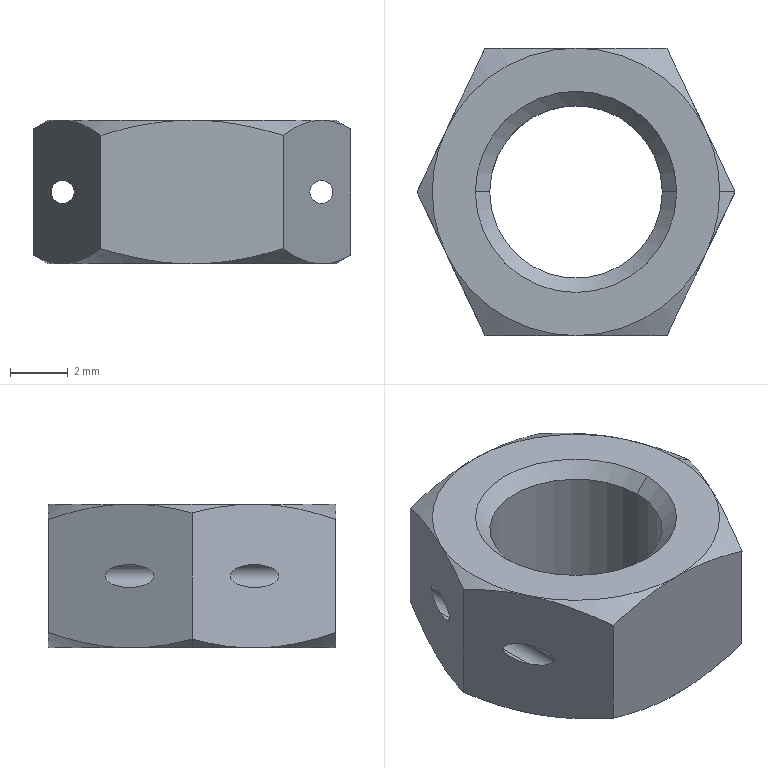Part | SolidWorks | features BaseBody 1 | 1 solid | 30 faces | box 11.062 x 10 x 5 mm | volume 284.112 mm3 | cone 16 | plane 8 | cylinder 6 | commonest cylinder face diameters 0.8 x4 6 x2
STEP:
#1=CARTESIAN_POINT('',(11.537,-31.104,-201.55));
#2=VERTEX_POINT('',#1);
#3=CARTESIAN_POINT('',(11.057,-28.966,-201.55));
#4=VERTEX_POINT('',#3);
#5=CARTESIAN_POINT('',(6.537,-31.104,-201.55));
#6=DIRECTION('',(0.,0.,1.));
#7=DIRECTION('',(-1.,0.,0.));
#8=AXIS2_PLACEMENT_3D('',#5,#6,#7);
#9=CIRCLE('',#8,5.);
#10=EDGE_CURVE('',#2,#4,#9,.T.);
#11=ORIENTED_EDGE('',*,*,#10,.F.);
#12=CARTESIAN_POINT('',(12.068,-31.104,-201.856));
#13=VERTEX_POINT('',#12);
#14=CARTESIAN_POINT('',(11.537,-31.104,-201.55));
#15=DIRECTION('',(0.866,0.,-0.5));
#16=VECTOR('',#15,1000.);
#17=LINE('',#14,#16);
#18=EDGE_CURVE('',#2,#13,#17,.T.);
#19=ORIENTED_EDGE('',*,*,#18,.T.);
#20=CARTESIAN_POINT('',(12.068,-31.104,-201.856));
#21=CARTESIAN_POINT('',(11.736,-30.402,-201.665));
#22=CARTESIAN_POINT('',(11.4,-29.691,-201.55));
#23=CARTESIAN_POINT('',(11.057,-28.966,-201.55));
#24=B_SPLINE_CURVE_WITH_KNOTS('',3,(#20,#21,#22,#23),.UNSPECIFIED.,.F.,.F.,(4,4),(0.,0.002384),.UNSPECIFIED.);
#25=EDGE_CURVE('',#13,#4,#24,.T.);
#26=ORIENTED_EDGE('',*,*,#25,.T.);
#27=EDGE_LOOP('',(#11,#19,#26));
#28=FACE_OUTER_BOUND('',#27,.T.);
#29=CARTESIAN_POINT('',(6.537,-31.104,-201.55));
#30=DIRECTION('',(0.,0.,-1.));
#31=DIRECTION('',(1.,0.,0.));
#32=AXIS2_PLACEMENT_3D('',#29,#30,#31);
#33=CONICAL_SURFACE('',#32,5.,1.047);
#34=ADVANCED_FACE('',(#28),#33,.T.);
#35=CARTESIAN_POINT('',(2.017,-28.966,-206.55));
#36=VERTEX_POINT('',#35);
#37=CARTESIAN_POINT('',(1.537,-31.104,-206.55));
#38=VERTEX_POINT('',#37);
#39=CARTESIAN_POINT('',(6.537,-31.104,-206.55));
#40=DIRECTION('',(0.,0.,1.));
#41=DIRECTION('',(-1.,0.,0.));
#42=AXIS2_PLACEMENT_3D('',#39,#40,#41);
#43=CIRCLE('',#42,5.);
#44=EDGE_CURVE('',#36,#38,#43,.T.);
#45=ORIENTED_EDGE('',*,*,#44,.T.);
#46=CARTESIAN_POINT('',(1.006,-31.104,-206.244));
#47=VERTEX_POINT('',#46);
#48=CARTESIAN_POINT('',(1.537,-31.104,-206.55));
#49=DIRECTION('',(-0.866,0.,0.5));
#50=VECTOR('',#49,1000.);
#51=LINE('',#48,#50);
#52=EDGE_CURVE('',#38,#47,#51,.T.);
#53=ORIENTED_EDGE('',*,*,#52,.T.);
#54=CARTESIAN_POINT('',(1.006,-31.104,-206.244));
#55=CARTESIAN_POINT('',(1.338,-30.402,-206.435));
#56=CARTESIAN_POINT('',(1.674,-29.691,-206.55));
#57=CARTESIAN_POINT('',(2.017,-28.966,-206.55));
#58=B_SPLINE_CURVE_WITH_KNOTS('',3,(#54,#55,#56,#57),.UNSPECIFIED.,.F.,.F.,(4,4),(0.,0.002384),.UNSPECIFIED.);
#59=EDGE_CURVE('',#47,#36,#58,.T.);
#60=ORIENTED_EDGE('',*,*,#59,.T.);
#61=EDGE_LOOP('',(#45,#53,#60));
#62=FACE_OUTER_BOUND('',#61,.T.);
#63=CARTESIAN_POINT('',(6.537,-31.104,-206.55));
#64=DIRECTION('',(0.,0.,1.));
#65=DIRECTION('',(-1.,0.,0.));
#66=AXIS2_PLACEMENT_3D('',#63,#64,#65);
#67=CONICAL_SURFACE('',#66,5.,1.047);
#68=ADVANCED_FACE('',(#62),#67,.T.);
#69=CARTESIAN_POINT('',(9.537,-31.104,-206.55));
#70=VERTEX_POINT('',#69);
#71=CARTESIAN_POINT('',(3.537,-31.104,-206.55));
#72=VERTEX_POINT('',#71);
#73=CARTESIAN_POINT('',(6.537,-31.104,-206.55));
#74=DIRECTION('',(0.,0.,-1.));
#75=DIRECTION('',(-1.,0.,0.));
#76=AXIS2_PLACEMENT_3D('',#73,#74,#75);
#77=CIRCLE('',#76,3.);
#78=EDGE_CURVE('',#70,#72,#77,.T.);
#79=ORIENTED_EDGE('',*,*,#78,.T.);
#80=CARTESIAN_POINT('',(3.537,-31.104,-202.05));
#81=VERTEX_POINT('',#80);
#82=CARTESIAN_POINT('',(3.537,-31.104,-211.55));
#83=DIRECTION('',(0.,0.,1.));
#84=VECTOR('',#83,1000.);
#85=LINE('',#82,#84);
#86=EDGE_CURVE('',#72,#81,#85,.T.);
#87=ORIENTED_EDGE('',*,*,#86,.T.);
#88=CARTESIAN_POINT('',(9.537,-31.104,-202.05));
#89=VERTEX_POINT('',#88);
#90=CARTESIAN_POINT('',(6.537,-31.104,-202.05));
#91=DIRECTION('',(0.,0.,1.));
#92=DIRECTION('',(-1.,0.,0.));
#93=AXIS2_PLACEMENT_3D('',#90,#91,#92);
#94=CIRCLE('',#93,3.);
#95=EDGE_CURVE('',#81,#89,#94,.T.);
#96=ORIENTED_EDGE('',*,*,#95,.T.);
#97=CARTESIAN_POINT('',(9.537,-31.104,-211.55));
#98=DIRECTION('',(0.,0.,1.));
#99=VECTOR('',#98,1000.);
#100=LINE('',#97,#99);
#101=EDGE_CURVE('',#70,#89,#100,.T.);
#102=ORIENTED_EDGE('',*,*,#101,.F.);
#103=EDGE_LOOP('',(#79,#87,#96,#102));
#104=FACE_OUTER_BOUND('',#103,.T.);
#105=CARTESIAN_POINT('',(6.537,-31.104,-211.55));
#106=DIRECTION('',(0.,0.,1.));
#107=DIRECTION('',(1.,0.,0.));
#108=AXIS2_PLACEMENT_3D('',#105,#106,#107);
#109=CYLINDRICAL_SURFACE('',#108,3.);
#110=ADVANCED_FACE('',(#104),#109,.F.);
#111=ORIENTED_EDGE('',*,*,#95,.F.);
#112=CARTESIAN_POINT('',(3.037,-31.104,-201.55));
#113=VERTEX_POINT('',#112);
#114=CARTESIAN_POINT('',(3.537,-31.104,-202.05));
#115=DIRECTION('',(-0.7071,0.,0.7071));
#116=VECTOR('',#115,1000.);
#117=LINE('',#114,#116);
#118=EDGE_CURVE('',#81,#113,#117,.T.);
#119=ORIENTED_EDGE('',*,*,#118,.T.);
#120=CARTESIAN_POINT('',(10.037,-31.104,-201.55));
#121=VERTEX_POINT('',#120);
#122=CARTESIAN_POINT('',(6.537,-31.104,-201.55));
#123=DIRECTION('',(0.,0.,-1.));
#124=DIRECTION('',(-1.,0.,0.));
#125=AXIS2_PLACEMENT_3D('',#122,#123,#124);
#126=CIRCLE('',#125,3.5);
#127=EDGE_CURVE('',#121,#113,#126,.T.);
#128=ORIENTED_EDGE('',*,*,#127,.F.);
#129=CARTESIAN_POINT('',(9.537,-31.104,-202.05));
#130=DIRECTION('',(0.7071,0.,0.7071));
#131=VECTOR('',#130,1000.);
#132=LINE('',#129,#131);
#133=EDGE_CURVE('',#89,#121,#132,.T.);
#134=ORIENTED_EDGE('',*,*,#133,.F.);
#135=EDGE_LOOP('',(#111,#119,#128,#134));
#136=FACE_OUTER_BOUND('',#135,.T.);
#137=CARTESIAN_POINT('',(6.537,-31.104,-202.05));
#138=DIRECTION('',(0.,0.,1.));
#139=DIRECTION('',(1.,0.,0.));
#140=AXIS2_PLACEMENT_3D('',#137,#138,#139);
#141=CONICAL_SURFACE('',#140,3.,0.7854);
#142=ADVANCED_FACE('',(#136),#141,.F.);
#143=CARTESIAN_POINT('',(11.037,-33.284,-204.45));
#144=VERTEX_POINT('',#143);
#145=CARTESIAN_POINT('',(11.037,-33.284,-203.65));
#146=VERTEX_POINT('',#145);
#147=CARTESIAN_POINT('',(11.037,-33.284,-204.45));
#148=CARTESIAN_POINT('',(10.237,-34.976,-204.45));
#149=CARTESIAN_POINT('',(10.237,-34.976,-203.65));
#150=CARTESIAN_POINT('',(11.037,-33.284,-203.65));
#151=(BOUNDED_CURVE()B_SPLINE_CURVE(3,(#147,#148,#149,#150),.UNSPECIFIED.,.F.,.T.)B_SPLINE_CURVE_WITH_KNOTS((4,4),(1.571,4.712),.UNSPECIFIED.)CURVE()GEOMETRIC_REPRESENTATION_ITEM()RATIONAL_B_SPLINE_CURVE((1.,0.3333,0.3333,1.))REPRESENTATION_ITEM(''));
#152=EDGE_CURVE('',#144,#146,#151,.T.);
#153=ORIENTED_EDGE('',*,*,#152,.F.);
#154=CARTESIAN_POINT('',(11.037,-28.924,-204.45));
#155=VERTEX_POINT('',#154);
#156=CARTESIAN_POINT('',(11.037,-36.104,-204.45));
#157=DIRECTION('',(0.,1.,0.));
#158=VECTOR('',#157,1000.);
#159=LINE('',#156,#158);
#160=EDGE_CURVE('',#144,#155,#159,.T.);
#161=ORIENTED_EDGE('',*,*,#160,.T.);
#162=CARTESIAN_POINT('',(11.037,-28.924,-203.65));
#163=VERTEX_POINT('',#162);
#164=CARTESIAN_POINT('',(11.037,-28.924,-203.65));
#165=CARTESIAN_POINT('',(10.237,-27.232,-203.65));
#166=CARTESIAN_POINT('',(10.237,-27.232,-204.45));
#167=CARTESIAN_POINT('',(11.037,-28.924,-204.45));
#168=(BOUNDED_CURVE()B_SPLINE_CURVE(3,(#164,#165,#166,#167),.UNSPECIFIED.,.F.,.T.)B_SPLINE_CURVE_WITH_KNOTS((4,4),(4.712,7.854),.UNSPECIFIED.)CURVE()GEOMETRIC_REPRESENTATION_ITEM()RATIONAL_B_SPLINE_CURVE((1.,0.3333,0.3333,1.))REPRESENTATION_ITEM(''));
#169=EDGE_CURVE('',#163,#155,#168,.T.);
#170=ORIENTED_EDGE('',*,*,#169,.F.);
#171=CARTESIAN_POINT('',(11.037,-36.104,-203.65));
#172=DIRECTION('',(0.,1.,0.));
#173=VECTOR('',#172,1000.);
#174=LINE('',#171,#173);
#175=EDGE_CURVE('',#146,#163,#174,.T.);
#176=ORIENTED_EDGE('',*,*,#175,.F.);
#177=EDGE_LOOP('',(#153,#161,#170,#176));
#178=FACE_OUTER_BOUND('',#177,.T.);
#179=CARTESIAN_POINT('',(11.037,-36.104,-204.05));
#180=DIRECTION('',(0.,1.,0.));
#181=DIRECTION('',(0.,0.,1.));
#182=AXIS2_PLACEMENT_3D('',#179,#180,#181);
#183=CYLINDRICAL_SURFACE('',#182,0.4);
#184=ADVANCED_FACE('',(#178),#183,.F.);
#185=CARTESIAN_POINT('',(2.037,-33.284,-204.45));
#186=VERTEX_POINT('',#185);
#187=CARTESIAN_POINT('',(2.037,-33.284,-203.65));
#188=VERTEX_POINT('',#187);
#189=CARTESIAN_POINT('',(2.037,-33.284,-204.45));
#190=CARTESIAN_POINT('',(1.237,-31.592,-204.45));
#191=CARTESIAN_POINT('',(1.237,-31.592,-203.65));
#192=CARTESIAN_POINT('',(2.037,-33.284,-203.65));
#193=(BOUNDED_CURVE()B_SPLINE_CURVE(3,(#189,#190,#191,#192),.UNSPECIFIED.,.F.,.F.)B_SPLINE_CURVE_WITH_KNOTS((4,4),(4.712,7.854),.UNSPECIFIED.)CURVE()GEOMETRIC_REPRESENTATION_ITEM()RATIONAL_B_SPLINE_CURVE((1.,0.3333,0.3333,1.))REPRESENTATION_ITEM(''));
#194=EDGE_CURVE('',#186,#188,#193,.T.);
#195=ORIENTED_EDGE('',*,*,#194,.F.);
#196=CARTESIAN_POINT('',(2.037,-28.924,-204.45));
#197=VERTEX_POINT('',#196);
#198=CARTESIAN_POINT('',(2.037,-36.104,-204.45));
#199=DIRECTION('',(0.,1.,0.));
#200=VECTOR('',#199,1000.);
#201=LINE('',#198,#200);
#202=EDGE_CURVE('',#186,#197,#201,.T.);
#203=ORIENTED_EDGE('',*,*,#202,.T.);
#204=CARTESIAN_POINT('',(2.037,-28.924,-203.65));
#205=VERTEX_POINT('',#204);
#206=CARTESIAN_POINT('',(2.037,-28.924,-203.65));
#207=CARTESIAN_POINT('',(1.237,-30.616,-203.65));
#208=CARTESIAN_POINT('',(1.237,-30.616,-204.45));
#209=CARTESIAN_POINT('',(2.037,-28.924,-204.45));
#210=(BOUNDED_CURVE()B_SPLINE_CURVE(3,(#206,#207,#208,#209),.UNSPECIFIED.,.F.,.F.)B_SPLINE_CURVE_WITH_KNOTS((4,4),(1.571,4.712),.UNSPECIFIED.)CURVE()GEOMETRIC_REPRESENTATION_ITEM()RATIONAL_B_SPLINE_CURVE((1.,0.3333,0.3333,1.))REPRESENTATION_ITEM(''));
#211=EDGE_CURVE('',#205,#197,#210,.T.);
#212=ORIENTED_EDGE('',*,*,#211,.F.);
#213=CARTESIAN_POINT('',(2.037,-36.104,-203.65));
#214=DIRECTION('',(0.,1.,0.));
#215=VECTOR('',#214,1000.);
#216=LINE('',#213,#215);
#217=EDGE_CURVE('',#188,#205,#216,.T.);
#218=ORIENTED_EDGE('',*,*,#217,.F.);
#219=EDGE_LOOP('',(#195,#203,#212,#218));
#220=FACE_OUTER_BOUND('',#219,.T.);
#221=CARTESIAN_POINT('',(2.037,-36.104,-204.05));
#222=DIRECTION('',(0.,1.,0.));
#223=DIRECTION('',(0.,0.,1.));
#224=AXIS2_PLACEMENT_3D('',#221,#222,#223);
#225=CYLINDRICAL_SURFACE('',#224,0.4);
#226=ADVANCED_FACE('',(#220),#225,.F.);
#227=ORIENTED_EDGE('',*,*,#202,.F.);
#228=CARTESIAN_POINT('',(2.037,-33.284,-203.65));
#229=CARTESIAN_POINT('',(2.837,-34.976,-203.65));
#230=CARTESIAN_POINT('',(2.837,-34.976,-204.45));
#231=CARTESIAN_POINT('',(2.037,-33.284,-204.45));
#232=(BOUNDED_CURVE()B_SPLINE_CURVE(3,(#228,#229,#230,#231),.UNSPECIFIED.,.F.,.F.)B_SPLINE_CURVE_WITH_KNOTS((4,4),(1.571,4.712),.UNSPECIFIED.)CURVE()GEOMETRIC_REPRESENTATION_ITEM()RATIONAL_B_SPLINE_CURVE((1.,0.3333,0.3333,1.))REPRESENTATION_ITEM(''));
#233=EDGE_CURVE('',#188,#186,#232,.T.);
#234=ORIENTED_EDGE('',*,*,#233,.F.);
#235=ORIENTED_EDGE('',*,*,#217,.T.);
#236=CARTESIAN_POINT('',(2.037,-28.924,-204.45));
#237=CARTESIAN_POINT('',(2.837,-27.232,-204.45));
#238=CARTESIAN_POINT('',(2.837,-27.232,-203.65));
#239=CARTESIAN_POINT('',(2.037,-28.924,-203.65));
#240=(BOUNDED_CURVE()B_SPLINE_CURVE(3,(#236,#237,#238,#239),.UNSPECIFIED.,.F.,.F.)B_SPLINE_CURVE_WITH_KNOTS((4,4),(4.712,7.854),.UNSPECIFIED.)CURVE()GEOMETRIC_REPRESENTATION_ITEM()RATIONAL_B_SPLINE_CURVE((1.,0.3333,0.3333,1.))REPRESENTATION_ITEM(''));
#241=EDGE_CURVE('',#197,#205,#240,.T.);
#242=ORIENTED_EDGE('',*,*,#241,.F.);
#243=EDGE_LOOP('',(#227,#234,#235,#242));
#244=FACE_OUTER_BOUND('',#243,.T.);
#245=CARTESIAN_POINT('',(2.037,-36.104,-204.05));
#246=DIRECTION('',(0.,1.,0.));
#247=DIRECTION('',(0.,0.,1.));
#248=AXIS2_PLACEMENT_3D('',#245,#246,#247);
#249=CYLINDRICAL_SURFACE('',#248,0.4);
#250=ADVANCED_FACE('',(#244),#249,.F.);
#251=ORIENTED_EDGE('',*,*,#160,.F.);
#252=CARTESIAN_POINT('',(11.037,-33.284,-203.65));
#253=CARTESIAN_POINT('',(11.837,-31.592,-203.65));
#254=CARTESIAN_POINT('',(11.837,-31.592,-204.45));
#255=CARTESIAN_POINT('',(11.037,-33.284,-204.45));
#256=(BOUNDED_CURVE()B_SPLINE_CURVE(3,(#252,#253,#254,#255),.UNSPECIFIED.,.F.,.T.)B_SPLINE_CURVE_WITH_KNOTS((4,4),(4.712,7.854),.UNSPECIFIED.)CURVE()GEOMETRIC_REPRESENTATION_ITEM()RATIONAL_B_SPLINE_CURVE((1.,0.3333,0.3333,1.))REPRESENTATION_ITEM(''));
#257=EDGE_CURVE('',#146,#144,#256,.T.);
#258=ORIENTED_EDGE('',*,*,#257,.F.);
#259=ORIENTED_EDGE('',*,*,#175,.T.);
#260=CARTESIAN_POINT('',(11.037,-28.924,-204.45));
#261=CARTESIAN_POINT('',(11.837,-30.616,-204.45));
#262=CARTESIAN_POINT('',(11.837,-30.616,-203.65));
#263=CARTESIAN_POINT('',(11.037,-28.924,-203.65));
#264=(BOUNDED_CURVE()B_SPLINE_CURVE(3,(#260,#261,#262,#263),.UNSPECIFIED.,.F.,.F.)B_SPLINE_CURVE_WITH_KNOTS((4,4),(1.571,4.712),.UNSPECIFIED.)CURVE()GEOMETRIC_REPRESENTATION_ITEM()RATIONAL_B_SPLINE_CURVE((1.,0.3333,0.3333,1.))REPRESENTATION_ITEM(''));
#265=EDGE_CURVE('',#155,#163,#264,.T.);
#266=ORIENTED_EDGE('',*,*,#265,.F.);
#267=EDGE_LOOP('',(#251,#258,#259,#266));
#268=FACE_OUTER_BOUND('',#267,.T.);
#269=CARTESIAN_POINT('',(11.037,-36.104,-204.05));
#270=DIRECTION('',(0.,1.,0.));
#271=DIRECTION('',(0.,0.,1.));
#272=AXIS2_PLACEMENT_3D('',#269,#270,#271);
#273=CYLINDRICAL_SURFACE('',#272,0.4);
#274=ADVANCED_FACE('',(#268),#273,.F.);
#275=ORIENTED_EDGE('',*,*,#118,.F.);
#276=CARTESIAN_POINT('',(6.537,-31.104,-202.05));
#277=DIRECTION('',(0.,0.,1.));
#278=DIRECTION('',(-1.,0.,0.));
#279=AXIS2_PLACEMENT_3D('',#276,#277,#278);
#280=CIRCLE('',#279,3.);
#281=EDGE_CURVE('',#89,#81,#280,.T.);
#282=ORIENTED_EDGE('',*,*,#281,.F.);
#283=ORIENTED_EDGE('',*,*,#133,.T.);
#284=CARTESIAN_POINT('',(6.537,-31.104,-201.55));
#285=DIRECTION('',(0.,0.,-1.));
#286=DIRECTION('',(-1.,0.,0.));
#287=AXIS2_PLACEMENT_3D('',#284,#285,#286);
#288=CIRCLE('',#287,3.5);
#289=EDGE_CURVE('',#113,#121,#288,.T.);
#290=ORIENTED_EDGE('',*,*,#289,.F.);
#291=EDGE_LOOP('',(#275,#282,#283,#290));
#292=FACE_OUTER_BOUND('',#291,.T.);
#293=CARTESIAN_POINT('',(6.537,-31.104,-202.05));
#294=DIRECTION('',(0.,0.,1.));
#295=DIRECTION('',(1.,0.,0.));
#296=AXIS2_PLACEMENT_3D('',#293,#294,#295);
#297=CONICAL_SURFACE('',#296,3.,0.7854);
#298=ADVANCED_FACE('',(#292),#297,.F.);
#299=ORIENTED_EDGE('',*,*,#86,.F.);
#300=CARTESIAN_POINT('',(6.537,-31.104,-206.55));
#301=DIRECTION('',(0.,0.,-1.));
#302=DIRECTION('',(-1.,0.,0.));
#303=AXIS2_PLACEMENT_3D('',#300,#301,#302);
#304=CIRCLE('',#303,3.);
#305=EDGE_CURVE('',#72,#70,#304,.T.);
#306=ORIENTED_EDGE('',*,*,#305,.T.);
#307=ORIENTED_EDGE('',*,*,#101,.T.);
#308=ORIENTED_EDGE('',*,*,#281,.T.);
#309=EDGE_LOOP('',(#299,#306,#307,#308));
#310=FACE_OUTER_BOUND('',#309,.T.);
#311=CARTESIAN_POINT('',(6.537,-31.104,-211.55));
#312=DIRECTION('',(0.,0.,1.));
#313=DIRECTION('',(1.,0.,0.));
#314=AXIS2_PLACEMENT_3D('',#311,#312,#313);
#315=CYLINDRICAL_SURFACE('',#314,3.);
#316=ADVANCED_FACE('',(#310),#315,.F.);
#317=CARTESIAN_POINT('',(2.017,-33.241,-206.55));
#318=VERTEX_POINT('',#317);
#319=CARTESIAN_POINT('',(6.537,-36.104,-206.55));
#320=VERTEX_POINT('',#319);
#321=CARTESIAN_POINT('',(6.537,-31.104,-206.55));
#322=DIRECTION('',(0.,0.,1.));
#323=DIRECTION('',(-1.,0.,0.));
#324=AXIS2_PLACEMENT_3D('',#321,#322,#323);
#325=CIRCLE('',#324,5.);
#326=EDGE_CURVE('',#318,#320,#325,.T.);
#327=ORIENTED_EDGE('',*,*,#326,.F.);
#328=CARTESIAN_POINT('',(6.537,-31.104,-206.55));
#329=DIRECTION('',(0.,0.,1.));
#330=DIRECTION('',(-1.,0.,0.));
#331=AXIS2_PLACEMENT_3D('',#328,#329,#330);
#332=CIRCLE('',#331,5.);
#333=EDGE_CURVE('',#38,#318,#332,.T.);
#334=ORIENTED_EDGE('',*,*,#333,.F.);
#335=ORIENTED_EDGE('',*,*,#44,.F.);
#336=CARTESIAN_POINT('',(6.537,-26.104,-206.55));
#337=VERTEX_POINT('',#336);
#338=CARTESIAN_POINT('',(6.537,-31.104,-206.55));
#339=DIRECTION('',(0.,0.,-1.));
#340=DIRECTION('',(-1.,0.,0.));
#341=AXIS2_PLACEMENT_3D('',#338,#339,#340);
#342=CIRCLE('',#341,5.);
#343=EDGE_CURVE('',#36,#337,#342,.T.);
#344=ORIENTED_EDGE('',*,*,#343,.T.);
#345=CARTESIAN_POINT('',(11.057,-28.966,-206.55));
#346=VERTEX_POINT('',#345);
#347=CARTESIAN_POINT('',(6.537,-31.104,-206.55));
#348=DIRECTION('',(0.,0.,1.));
#349=DIRECTION('',(-1.,0.,0.));
#350=AXIS2_PLACEMENT_3D('',#347,#348,#349);
#351=CIRCLE('',#350,5.);
#352=EDGE_CURVE('',#346,#337,#351,.T.);
#353=ORIENTED_EDGE('',*,*,#352,.F.);
#354=CARTESIAN_POINT('',(11.057,-33.241,-206.55));
#355=VERTEX_POINT('',#354);
#356=CARTESIAN_POINT('',(6.537,-31.104,-206.55));
#357=DIRECTION('',(0.,0.,1.));
#358=DIRECTION('',(-1.,0.,0.));
#359=AXIS2_PLACEMENT_3D('',#356,#357,#358);
#360=CIRCLE('',#359,5.);
#361=EDGE_CURVE('',#355,#346,#360,.T.);
#362=ORIENTED_EDGE('',*,*,#361,.F.);
#363=CARTESIAN_POINT('',(6.537,-31.104,-206.55));
#364=DIRECTION('',(0.,0.,1.));
#365=DIRECTION('',(-1.,0.,0.));
#366=AXIS2_PLACEMENT_3D('',#363,#364,#365);
#367=CIRCLE('',#366,5.);
#368=EDGE_CURVE('',#320,#355,#367,.T.);
#369=ORIENTED_EDGE('',*,*,#368,.F.);
#370=EDGE_LOOP('',(#327,#334,#335,#344,#353,#362,#369));
#371=FACE_OUTER_BOUND('',#370,.T.);
#372=ORIENTED_EDGE('',*,*,#78,.F.);
#373=ORIENTED_EDGE('',*,*,#305,.F.);
#374=EDGE_LOOP('',(#372,#373));
#375=FACE_BOUND('',#374,.T.);
#376=CARTESIAN_POINT('',(14.432,-26.104,-206.55));
#377=DIRECTION('',(0.,0.,-1.));
#378=DIRECTION('',(0.,-1.,0.));
#379=AXIS2_PLACEMENT_3D('',#376,#377,#378);
#380=PLANE('',#379);
#381=ADVANCED_FACE('',(#371,#375),#380,.T.);
#382=CARTESIAN_POINT('',(3.371,-36.104,-206.02));
#383=VERTEX_POINT('',#382);
#384=CARTESIAN_POINT('',(3.371,-36.104,-206.02));
#385=CARTESIAN_POINT('',(2.93,-35.171,-206.338));
#386=CARTESIAN_POINT('',(2.481,-34.222,-206.55));
#387=CARTESIAN_POINT('',(2.017,-33.241,-206.55));
#388=B_SPLINE_CURVE_WITH_KNOTS('',3,(#384,#385,#386,#387),.UNSPECIFIED.,.F.,.F.,(4,4),(0.,0.003211),.UNSPECIFIED.);
#389=EDGE_CURVE('',#383,#318,#388,.T.);
#390=ORIENTED_EDGE('',*,*,#389,.T.);
#391=ORIENTED_EDGE('',*,*,#326,.T.);
#392=CARTESIAN_POINT('',(6.537,-36.104,-206.55));
#393=CARTESIAN_POINT('',(5.452,-36.104,-206.55));
#394=CARTESIAN_POINT('',(4.402,-36.104,-206.338));
#395=CARTESIAN_POINT('',(3.371,-36.104,-206.02));
#396=B_SPLINE_CURVE_WITH_KNOTS('',3,(#392,#393,#394,#395),.UNSPECIFIED.,.F.,.F.,(4,4),(0.,0.003211),.UNSPECIFIED.);
#397=EDGE_CURVE('',#320,#383,#396,.T.);
#398=ORIENTED_EDGE('',*,*,#397,.T.);
#399=EDGE_LOOP('',(#390,#391,#398));
#400=FACE_OUTER_BOUND('',#399,.T.);
#401=CARTESIAN_POINT('',(6.537,-31.104,-206.55));
#402=DIRECTION('',(0.,0.,1.));
#403=DIRECTION('',(-1.,0.,0.));
#404=AXIS2_PLACEMENT_3D('',#401,#402,#403);
#405=CONICAL_SURFACE('',#404,5.,1.047);
#406=ADVANCED_FACE('',(#400),#405,.T.);
#407=CARTESIAN_POINT('',(9.704,-36.104,-206.02));
#408=VERTEX_POINT('',#407);
#409=CARTESIAN_POINT('',(11.057,-33.241,-206.55));
#410=CARTESIAN_POINT('',(10.593,-34.222,-206.55));
#411=CARTESIAN_POINT('',(10.145,-35.171,-206.338));
#412=CARTESIAN_POINT('',(9.704,-36.104,-206.02));
#413=B_SPLINE_CURVE_WITH_KNOTS('',3,(#409,#410,#411,#412),.UNSPECIFIED.,.F.,.F.,(4,4),(0.,0.003211),.UNSPECIFIED.);
#414=EDGE_CURVE('',#355,#408,#413,.T.);
#415=ORIENTED_EDGE('',*,*,#414,.T.);
#416=CARTESIAN_POINT('',(9.704,-36.104,-206.02));
#417=CARTESIAN_POINT('',(8.672,-36.104,-206.338));
#418=CARTESIAN_POINT('',(7.622,-36.104,-206.55));
#419=CARTESIAN_POINT('',(6.537,-36.104,-206.55));
#420=B_SPLINE_CURVE_WITH_KNOTS('',3,(#416,#417,#418,#419),.UNSPECIFIED.,.F.,.F.,(4,4),(0.,0.003211),.UNSPECIFIED.);
#421=EDGE_CURVE('',#408,#320,#420,.T.);
#422=ORIENTED_EDGE('',*,*,#421,.T.);
#423=ORIENTED_EDGE('',*,*,#368,.T.);
#424=EDGE_LOOP('',(#415,#422,#423));
#425=FACE_OUTER_BOUND('',#424,.T.);
#426=CARTESIAN_POINT('',(6.537,-31.104,-206.55));
#427=DIRECTION('',(0.,0.,1.));
#428=DIRECTION('',(-1.,0.,0.));
#429=AXIS2_PLACEMENT_3D('',#426,#427,#428);
#430=CONICAL_SURFACE('',#429,5.,1.047);
#431=ADVANCED_FACE('',(#425),#430,.T.);
#432=CARTESIAN_POINT('',(12.068,-31.104,-206.244));
#433=VERTEX_POINT('',#432);
#434=CARTESIAN_POINT('',(11.057,-28.966,-206.55));
#435=CARTESIAN_POINT('',(11.4,-29.691,-206.55));
#436=CARTESIAN_POINT('',(11.736,-30.402,-206.435));
#437=CARTESIAN_POINT('',(12.068,-31.104,-206.244));
#438=B_SPLINE_CURVE_WITH_KNOTS('',3,(#434,#435,#436,#437),.UNSPECIFIED.,.F.,.F.,(4,4),(0.,0.002384),.UNSPECIFIED.);
#439=EDGE_CURVE('',#346,#433,#438,.T.);
#440=ORIENTED_EDGE('',*,*,#439,.T.);
#441=CARTESIAN_POINT('',(12.068,-31.104,-206.244));
#442=CARTESIAN_POINT('',(11.736,-31.806,-206.435));
#443=CARTESIAN_POINT('',(11.4,-32.517,-206.55));
#444=CARTESIAN_POINT('',(11.057,-33.241,-206.55));
#445=B_SPLINE_CURVE_WITH_KNOTS('',3,(#441,#442,#443,#444),.UNSPECIFIED.,.F.,.F.,(4,4),(0.,0.002384),.UNSPECIFIED.);
#446=EDGE_CURVE('',#433,#355,#445,.T.);
#447=ORIENTED_EDGE('',*,*,#446,.T.);
#448=ORIENTED_EDGE('',*,*,#361,.T.);
#449=EDGE_LOOP('',(#440,#447,#448));
#450=FACE_OUTER_BOUND('',#449,.T.);
#451=CARTESIAN_POINT('',(6.537,-31.104,-206.55));
#452=DIRECTION('',(0.,0.,1.));
#453=DIRECTION('',(-1.,0.,0.));
#454=AXIS2_PLACEMENT_3D('',#451,#452,#453);
#455=CONICAL_SURFACE('',#454,5.,1.047);
#456=ADVANCED_FACE('',(#450),#455,.T.);
#457=CARTESIAN_POINT('',(9.704,-26.104,-206.02));
#458=VERTEX_POINT('',#457);
#459=CARTESIAN_POINT('',(6.537,-26.104,-206.55));
#460=CARTESIAN_POINT('',(7.622,-26.104,-206.55));
#461=CARTESIAN_POINT('',(8.672,-26.104,-206.338));
#462=CARTESIAN_POINT('',(9.704,-26.104,-206.02));
#463=B_SPLINE_CURVE_WITH_KNOTS('',3,(#459,#460,#461,#462),.UNSPECIFIED.,.F.,.F.,(4,4),(0.,0.003211),.UNSPECIFIED.);
#464=EDGE_CURVE('',#337,#458,#463,.T.);
#465=ORIENTED_EDGE('',*,*,#464,.T.);
#466=CARTESIAN_POINT('',(9.704,-26.104,-206.02));
#467=CARTESIAN_POINT('',(10.145,-27.037,-206.338));
#468=CARTESIAN_POINT('',(10.593,-27.985,-206.55));
#469=CARTESIAN_POINT('',(11.057,-28.966,-206.55));
#470=B_SPLINE_CURVE_WITH_KNOTS('',3,(#466,#467,#468,#469),.UNSPECIFIED.,.F.,.F.,(4,4),(0.,0.003211),.UNSPECIFIED.);
#471=EDGE_CURVE('',#458,#346,#470,.T.);
#472=ORIENTED_EDGE('',*,*,#471,.T.);
#473=ORIENTED_EDGE('',*,*,#352,.T.);
#474=EDGE_LOOP('',(#465,#472,#473));
#475=FACE_OUTER_BOUND('',#474,.T.);
#476=CARTESIAN_POINT('',(6.537,-31.104,-206.55));
#477=DIRECTION('',(0.,0.,1.));
#478=DIRECTION('',(-1.,0.,0.));
#479=AXIS2_PLACEMENT_3D('',#476,#477,#478);
#480=CONICAL_SURFACE('',#479,5.,1.047);
#481=ADVANCED_FACE('',(#475),#480,.T.);
#482=CARTESIAN_POINT('',(3.371,-26.104,-206.02));
#483=VERTEX_POINT('',#482);
#484=CARTESIAN_POINT('',(3.371,-26.104,-206.02));
#485=CARTESIAN_POINT('',(4.402,-26.104,-206.338));
#486=CARTESIAN_POINT('',(5.452,-26.104,-206.55));
#487=CARTESIAN_POINT('',(6.537,-26.104,-206.55));
#488=B_SPLINE_CURVE_WITH_KNOTS('',3,(#484,#485,#486,#487),.UNSPECIFIED.,.F.,.F.,(4,4),(0.,0.003211),.UNSPECIFIED.);
#489=EDGE_CURVE('',#483,#337,#488,.T.);
#490=ORIENTED_EDGE('',*,*,#489,.T.);
#491=ORIENTED_EDGE('',*,*,#343,.F.);
#492=CARTESIAN_POINT('',(2.017,-28.966,-206.55));
#493=CARTESIAN_POINT('',(2.481,-27.985,-206.55));
#494=CARTESIAN_POINT('',(2.93,-27.037,-206.338));
#495=CARTESIAN_POINT('',(3.371,-26.104,-206.02));
#496=B_SPLINE_CURVE_WITH_KNOTS('',3,(#492,#493,#494,#495),.UNSPECIFIED.,.F.,.F.,(4,4),(0.,0.003211),.UNSPECIFIED.);
#497=EDGE_CURVE('',#36,#483,#496,.T.);
#498=ORIENTED_EDGE('',*,*,#497,.T.);
#499=EDGE_LOOP('',(#490,#491,#498));
#500=FACE_OUTER_BOUND('',#499,.T.);
#501=CARTESIAN_POINT('',(6.537,-31.104,-206.55));
#502=DIRECTION('',(0.,0.,1.));
#503=DIRECTION('',(-1.,0.,0.));
#504=AXIS2_PLACEMENT_3D('',#501,#502,#503);
#505=CONICAL_SURFACE('',#504,5.,1.047);
#506=ADVANCED_FACE('',(#500),#505,.T.);
#507=ORIENTED_EDGE('',*,*,#52,.F.);
#508=ORIENTED_EDGE('',*,*,#333,.T.);
#509=CARTESIAN_POINT('',(2.017,-33.241,-206.55));
#510=CARTESIAN_POINT('',(1.674,-32.517,-206.55));
#511=CARTESIAN_POINT('',(1.338,-31.806,-206.435));
#512=CARTESIAN_POINT('',(1.006,-31.104,-206.244));
#513=B_SPLINE_CURVE_WITH_KNOTS('',3,(#509,#510,#511,#512),.UNSPECIFIED.,.F.,.F.,(4,4),(0.,0.002384),.UNSPECIFIED.);
#514=EDGE_CURVE('',#318,#47,#513,.T.);
#515=ORIENTED_EDGE('',*,*,#514,.T.);
#516=EDGE_LOOP('',(#507,#508,#515));
#517=FACE_OUTER_BOUND('',#516,.T.);
#518=CARTESIAN_POINT('',(6.537,-31.104,-206.55));
#519=DIRECTION('',(0.,0.,1.));
#520=DIRECTION('',(-1.,0.,0.));
#521=AXIS2_PLACEMENT_3D('',#518,#519,#520);
#522=CONICAL_SURFACE('',#521,5.,1.047);
#523=ADVANCED_FACE('',(#517),#522,.T.);
#524=CARTESIAN_POINT('',(2.017,-28.966,-201.55));
#525=VERTEX_POINT('',#524);
#526=CARTESIAN_POINT('',(2.017,-33.241,-201.55));
#527=VERTEX_POINT('',#526);
#528=CARTESIAN_POINT('',(6.537,-31.104,-201.55));
#529=DIRECTION('',(0.,0.,1.));
#530=DIRECTION('',(-1.,0.,0.));
#531=AXIS2_PLACEMENT_3D('',#528,#529,#530);
#532=CIRCLE('',#531,5.);
#533=EDGE_CURVE('',#525,#527,#532,.T.);
#534=ORIENTED_EDGE('',*,*,#533,.T.);
#535=CARTESIAN_POINT('',(6.537,-36.104,-201.55));
#536=VERTEX_POINT('',#535);
#537=CARTESIAN_POINT('',(6.537,-31.104,-201.55));
#538=DIRECTION('',(0.,0.,1.));
#539=DIRECTION('',(-1.,0.,0.));
#540=AXIS2_PLACEMENT_3D('',#537,#538,#539);
#541=CIRCLE('',#540,5.);
#542=EDGE_CURVE('',#527,#536,#541,.T.);
#543=ORIENTED_EDGE('',*,*,#542,.T.);
#544=CARTESIAN_POINT('',(11.057,-33.241,-201.55));
#545=VERTEX_POINT('',#544);
#546=CARTESIAN_POINT('',(6.537,-31.104,-201.55));
#547=DIRECTION('',(0.,0.,1.));
#548=DIRECTION('',(-1.,0.,0.));
#549=AXIS2_PLACEMENT_3D('',#546,#547,#548);
#550=CIRCLE('',#549,5.);
#551=EDGE_CURVE('',#536,#545,#550,.T.);
#552=ORIENTED_EDGE('',*,*,#551,.T.);
#553=CARTESIAN_POINT('',(6.537,-31.104,-201.55));
#554=DIRECTION('',(0.,0.,1.));
#555=DIRECTION('',(-1.,0.,0.));
#556=AXIS2_PLACEMENT_3D('',#553,#554,#555);
#557=CIRCLE('',#556,5.);
#558=EDGE_CURVE('',#545,#2,#557,.T.);
#559=ORIENTED_EDGE('',*,*,#558,.T.);
#560=ORIENTED_EDGE('',*,*,#10,.T.);
#561=CARTESIAN_POINT('',(6.537,-26.104,-201.55));
#562=VERTEX_POINT('',#561);
#563=CARTESIAN_POINT('',(6.537,-31.104,-201.55));
#564=DIRECTION('',(0.,0.,1.));
#565=DIRECTION('',(1.,0.,0.));
#566=AXIS2_PLACEMENT_3D('',#563,#564,#565);
#567=CIRCLE('',#566,5.);
#568=EDGE_CURVE('',#4,#562,#567,.T.);
#569=ORIENTED_EDGE('',*,*,#568,.T.);
#570=CARTESIAN_POINT('',(6.537,-31.104,-201.55));
#571=DIRECTION('',(0.,0.,1.));
#572=DIRECTION('',(-1.,0.,0.));
#573=AXIS2_PLACEMENT_3D('',#570,#571,#572);
#574=CIRCLE('',#573,5.);
#575=EDGE_CURVE('',#562,#525,#574,.T.);
#576=ORIENTED_EDGE('',*,*,#575,.T.);
#577=EDGE_LOOP('',(#534,#543,#552,#559,#560,#569,#576));
#578=FACE_OUTER_BOUND('',#577,.T.);
#579=ORIENTED_EDGE('',*,*,#127,.T.);
#580=ORIENTED_EDGE('',*,*,#289,.T.);
#581=EDGE_LOOP('',(#579,#580));
#582=FACE_BOUND('',#581,.T.);
#583=CARTESIAN_POINT('',(14.432,-26.104,-201.55));
#584=DIRECTION('',(0.,0.,-1.));
#585=DIRECTION('',(0.,-1.,0.));
#586=AXIS2_PLACEMENT_3D('',#583,#584,#585);
#587=PLANE('',#586);
#588=ADVANCED_FACE('',(#578,#582),#587,.F.);
#589=CARTESIAN_POINT('',(3.371,-36.104,-202.08));
#590=VERTEX_POINT('',#589);
#591=CARTESIAN_POINT('',(2.017,-33.241,-201.55));
#592=CARTESIAN_POINT('',(2.481,-34.222,-201.55));
#593=CARTESIAN_POINT('',(2.93,-35.171,-201.762));
#594=CARTESIAN_POINT('',(3.371,-36.104,-202.08));
#595=B_SPLINE_CURVE_WITH_KNOTS('',3,(#591,#592,#593,#594),.UNSPECIFIED.,.F.,.F.,(4,4),(0.,0.003211),.UNSPECIFIED.);
#596=EDGE_CURVE('',#527,#590,#595,.T.);
#597=ORIENTED_EDGE('',*,*,#596,.T.);
#598=CARTESIAN_POINT('',(3.371,-36.104,-202.08));
#599=CARTESIAN_POINT('',(4.402,-36.104,-201.762));
#600=CARTESIAN_POINT('',(5.452,-36.104,-201.55));
#601=CARTESIAN_POINT('',(6.537,-36.104,-201.55));
#602=B_SPLINE_CURVE_WITH_KNOTS('',3,(#598,#599,#600,#601),.UNSPECIFIED.,.F.,.F.,(4,4),(0.,0.003211),.UNSPECIFIED.);
#603=EDGE_CURVE('',#590,#536,#602,.T.);
#604=ORIENTED_EDGE('',*,*,#603,.T.);
#605=ORIENTED_EDGE('',*,*,#542,.F.);
#606=EDGE_LOOP('',(#597,#604,#605));
#607=FACE_OUTER_BOUND('',#606,.T.);
#608=CARTESIAN_POINT('',(6.537,-31.104,-201.55));
#609=DIRECTION('',(0.,0.,-1.));
#610=DIRECTION('',(1.,0.,0.));
#611=AXIS2_PLACEMENT_3D('',#608,#609,#610);
#612=CONICAL_SURFACE('',#611,5.,1.047);
#613=ADVANCED_FACE('',(#607),#612,.T.);
#614=CARTESIAN_POINT('',(9.704,-36.104,-202.08));
#615=VERTEX_POINT('',#614);
#616=CARTESIAN_POINT('',(9.704,-36.104,-202.08));
#617=CARTESIAN_POINT('',(10.145,-35.171,-201.762));
#618=CARTESIAN_POINT('',(10.593,-34.222,-201.55));
#619=CARTESIAN_POINT('',(11.057,-33.241,-201.55));
#620=B_SPLINE_CURVE_WITH_KNOTS('',3,(#616,#617,#618,#619),.UNSPECIFIED.,.F.,.F.,(4,4),(0.,0.003211),.UNSPECIFIED.);
#621=EDGE_CURVE('',#615,#545,#620,.T.);
#622=ORIENTED_EDGE('',*,*,#621,.T.);
#623=ORIENTED_EDGE('',*,*,#551,.F.);
#624=CARTESIAN_POINT('',(6.537,-36.104,-201.55));
#625=CARTESIAN_POINT('',(7.622,-36.104,-201.55));
#626=CARTESIAN_POINT('',(8.672,-36.104,-201.762));
#627=CARTESIAN_POINT('',(9.704,-36.104,-202.08));
#628=B_SPLINE_CURVE_WITH_KNOTS('',3,(#624,#625,#626,#627),.UNSPECIFIED.,.F.,.F.,(4,4),(0.,0.003211),.UNSPECIFIED.);
#629=EDGE_CURVE('',#536,#615,#628,.T.);
#630=ORIENTED_EDGE('',*,*,#629,.T.);
#631=EDGE_LOOP('',(#622,#623,#630));
#632=FACE_OUTER_BOUND('',#631,.T.);
#633=CARTESIAN_POINT('',(6.537,-31.104,-201.55));
#634=DIRECTION('',(0.,0.,-1.));
#635=DIRECTION('',(1.,0.,0.));
#636=AXIS2_PLACEMENT_3D('',#633,#634,#635);
#637=CONICAL_SURFACE('',#636,5.,1.047);
#638=ADVANCED_FACE('',(#632),#637,.T.);
#639=ORIENTED_EDGE('',*,*,#18,.F.);
#640=ORIENTED_EDGE('',*,*,#558,.F.);
#641=CARTESIAN_POINT('',(11.057,-33.241,-201.55));
#642=CARTESIAN_POINT('',(11.4,-32.517,-201.55));
#643=CARTESIAN_POINT('',(11.736,-31.806,-201.665));
#644=CARTESIAN_POINT('',(12.068,-31.104,-201.856));
#645=B_SPLINE_CURVE_WITH_KNOTS('',3,(#641,#642,#643,#644),.UNSPECIFIED.,.F.,.F.,(4,4),(0.,0.002384),.UNSPECIFIED.);
#646=EDGE_CURVE('',#545,#13,#645,.T.);
#647=ORIENTED_EDGE('',*,*,#646,.T.);
#648=EDGE_LOOP('',(#639,#640,#647));
#649=FACE_OUTER_BOUND('',#648,.T.);
#650=CARTESIAN_POINT('',(6.537,-31.104,-201.55));
#651=DIRECTION('',(0.,0.,-1.));
#652=DIRECTION('',(1.,0.,0.));
#653=AXIS2_PLACEMENT_3D('',#650,#651,#652);
#654=CONICAL_SURFACE('',#653,5.,1.047);
#655=ADVANCED_FACE('',(#649),#654,.T.);
#656=CARTESIAN_POINT('',(9.704,-26.104,-202.08));
#657=VERTEX_POINT('',#656);
#658=CARTESIAN_POINT('',(11.057,-28.966,-201.55));
#659=CARTESIAN_POINT('',(10.593,-27.985,-201.55));
#660=CARTESIAN_POINT('',(10.145,-27.037,-201.762));
#661=CARTESIAN_POINT('',(9.704,-26.104,-202.08));
#662=B_SPLINE_CURVE_WITH_KNOTS('',3,(#658,#659,#660,#661),.UNSPECIFIED.,.F.,.F.,(4,4),(0.,0.003211),.UNSPECIFIED.);
#663=EDGE_CURVE('',#4,#657,#662,.T.);
#664=ORIENTED_EDGE('',*,*,#663,.T.);
#665=CARTESIAN_POINT('',(9.704,-26.104,-202.08));
#666=CARTESIAN_POINT('',(8.672,-26.104,-201.762));
#667=CARTESIAN_POINT('',(7.622,-26.104,-201.55));
#668=CARTESIAN_POINT('',(6.537,-26.104,-201.55));
#669=B_SPLINE_CURVE_WITH_KNOTS('',3,(#665,#666,#667,#668),.UNSPECIFIED.,.F.,.F.,(4,4),(0.,0.003211),.UNSPECIFIED.);
#670=EDGE_CURVE('',#657,#562,#669,.T.);
#671=ORIENTED_EDGE('',*,*,#670,.T.);
#672=ORIENTED_EDGE('',*,*,#568,.F.);
#673=EDGE_LOOP('',(#664,#671,#672));
#674=FACE_OUTER_BOUND('',#673,.T.);
#675=CARTESIAN_POINT('',(6.537,-31.104,-201.55));
#676=DIRECTION('',(0.,0.,-1.));
#677=DIRECTION('',(1.,0.,0.));
#678=AXIS2_PLACEMENT_3D('',#675,#676,#677);
#679=CONICAL_SURFACE('',#678,5.,1.047);
#680=ADVANCED_FACE('',(#674),#679,.T.);
#681=CARTESIAN_POINT('',(3.371,-26.104,-202.08));
#682=VERTEX_POINT('',#681);
#683=CARTESIAN_POINT('',(6.537,-26.104,-201.55));
#684=CARTESIAN_POINT('',(5.452,-26.104,-201.55));
#685=CARTESIAN_POINT('',(4.402,-26.104,-201.762));
#686=CARTESIAN_POINT('',(3.371,-26.104,-202.08));
#687=B_SPLINE_CURVE_WITH_KNOTS('',3,(#683,#684,#685,#686),.UNSPECIFIED.,.F.,.F.,(4,4),(0.,0.003211),.UNSPECIFIED.);
#688=EDGE_CURVE('',#562,#682,#687,.T.);
#689=ORIENTED_EDGE('',*,*,#688,.T.);
#690=CARTESIAN_POINT('',(3.371,-26.104,-202.08));
#691=CARTESIAN_POINT('',(2.93,-27.037,-201.762));
#692=CARTESIAN_POINT('',(2.481,-27.985,-201.55));
#693=CARTESIAN_POINT('',(2.017,-28.966,-201.55));
#694=B_SPLINE_CURVE_WITH_KNOTS('',3,(#690,#691,#692,#693),.UNSPECIFIED.,.F.,.F.,(4,4),(0.,0.003211),.UNSPECIFIED.);
#695=EDGE_CURVE('',#682,#525,#694,.T.);
#696=ORIENTED_EDGE('',*,*,#695,.T.);
#697=ORIENTED_EDGE('',*,*,#575,.F.);
#698=EDGE_LOOP('',(#689,#696,#697));
#699=FACE_OUTER_BOUND('',#698,.T.);
#700=CARTESIAN_POINT('',(6.537,-31.104,-201.55));
#701=DIRECTION('',(0.,0.,-1.));
#702=DIRECTION('',(1.,0.,0.));
#703=AXIS2_PLACEMENT_3D('',#700,#701,#702);
#704=CONICAL_SURFACE('',#703,5.,1.047);
#705=ADVANCED_FACE('',(#699),#704,.T.);
#706=CARTESIAN_POINT('',(1.006,-31.104,-201.856));
#707=VERTEX_POINT('',#706);
#708=CARTESIAN_POINT('',(2.017,-28.966,-201.55));
#709=CARTESIAN_POINT('',(1.674,-29.691,-201.55));
#710=CARTESIAN_POINT('',(1.338,-30.402,-201.665));
#711=CARTESIAN_POINT('',(1.006,-31.104,-201.856));
#712=B_SPLINE_CURVE_WITH_KNOTS('',3,(#708,#709,#710,#711),.UNSPECIFIED.,.F.,.F.,(4,4),(0.,0.002384),.UNSPECIFIED.);
#713=EDGE_CURVE('',#525,#707,#712,.T.);
#714=ORIENTED_EDGE('',*,*,#713,.T.);
#715=CARTESIAN_POINT('',(1.006,-31.104,-201.856));
#716=CARTESIAN_POINT('',(1.338,-31.806,-201.665));
#717=CARTESIAN_POINT('',(1.674,-32.517,-201.55));
#718=CARTESIAN_POINT('',(2.017,-33.241,-201.55));
#719=B_SPLINE_CURVE_WITH_KNOTS('',3,(#715,#716,#717,#718),.UNSPECIFIED.,.F.,.F.,(4,4),(0.,0.002384),.UNSPECIFIED.);
#720=EDGE_CURVE('',#707,#527,#719,.T.);
#721=ORIENTED_EDGE('',*,*,#720,.T.);
#722=ORIENTED_EDGE('',*,*,#533,.F.);
#723=EDGE_LOOP('',(#714,#721,#722));
#724=FACE_OUTER_BOUND('',#723,.T.);
#725=CARTESIAN_POINT('',(6.537,-31.104,-201.55));
#726=DIRECTION('',(0.,0.,-1.));
#727=DIRECTION('',(1.,0.,0.));
#728=AXIS2_PLACEMENT_3D('',#725,#726,#727);
#729=CONICAL_SURFACE('',#728,5.,1.047);
#730=ADVANCED_FACE('',(#724),#729,.T.);
#731=ORIENTED_EDGE('',*,*,#421,.F.);
#732=CARTESIAN_POINT('',(9.704,-36.104,-201.55));
#733=DIRECTION('',(0.,0.,-1.));
#734=VECTOR('',#733,1000.);
#735=LINE('',#732,#734);
#736=EDGE_CURVE('',#615,#408,#735,.T.);
#737=ORIENTED_EDGE('',*,*,#736,.F.);
#738=ORIENTED_EDGE('',*,*,#629,.F.);
#739=ORIENTED_EDGE('',*,*,#603,.F.);
#740=CARTESIAN_POINT('',(3.371,-36.104,-201.55));
#741=DIRECTION('',(0.,0.,-1.));
#742=VECTOR('',#741,1000.);
#743=LINE('',#740,#742);
#744=EDGE_CURVE('',#590,#383,#743,.T.);
#745=ORIENTED_EDGE('',*,*,#744,.T.);
#746=ORIENTED_EDGE('',*,*,#397,.F.);
#747=EDGE_LOOP('',(#731,#737,#738,#739,#745,#746));
#748=FACE_OUTER_BOUND('',#747,.T.);
#749=CARTESIAN_POINT('',(3.371,-36.104,-201.55));
#750=DIRECTION('',(0.,1.,0.));
#751=DIRECTION('',(1.,0.,0.));
#752=AXIS2_PLACEMENT_3D('',#749,#750,#751);
#753=PLANE('',#752);
#754=ADVANCED_FACE('',(#748),#753,.F.);
#755=ORIENTED_EDGE('',*,*,#389,.F.);
#756=ORIENTED_EDGE('',*,*,#744,.F.);
#757=ORIENTED_EDGE('',*,*,#596,.F.);
#758=ORIENTED_EDGE('',*,*,#720,.F.);
#759=CARTESIAN_POINT('',(1.006,-31.104,-201.55));
#760=DIRECTION('',(0.,0.,-1.));
#761=VECTOR('',#760,1000.);
#762=LINE('',#759,#761);
#763=EDGE_CURVE('',#707,#47,#762,.T.);
#764=ORIENTED_EDGE('',*,*,#763,.T.);
#765=ORIENTED_EDGE('',*,*,#514,.F.);
#766=EDGE_LOOP('',(#755,#756,#757,#758,#764,#765));
#767=FACE_OUTER_BOUND('',#766,.T.);
#768=ORIENTED_EDGE('',*,*,#233,.T.);
#769=ORIENTED_EDGE('',*,*,#194,.T.);
#770=EDGE_LOOP('',(#768,#769));
#771=FACE_BOUND('',#770,.T.);
#772=CARTESIAN_POINT('',(3.371,-36.104,-201.55));
#773=DIRECTION('',(0.904,0.4275,0.));
#774=DIRECTION('',(0.,0.,-1.));
#775=AXIS2_PLACEMENT_3D('',#772,#773,#774);
#776=PLANE('',#775);
#777=ADVANCED_FACE('',(#767,#771),#776,.F.);
#778=ORIENTED_EDGE('',*,*,#59,.F.);
#779=ORIENTED_EDGE('',*,*,#763,.F.);
#780=ORIENTED_EDGE('',*,*,#713,.F.);
#781=ORIENTED_EDGE('',*,*,#695,.F.);
#782=CARTESIAN_POINT('',(3.371,-26.104,-201.55));
#783=DIRECTION('',(0.,0.,-1.));
#784=VECTOR('',#783,1000.);
#785=LINE('',#782,#784);
#786=EDGE_CURVE('',#682,#483,#785,.T.);
#787=ORIENTED_EDGE('',*,*,#786,.T.);
#788=ORIENTED_EDGE('',*,*,#497,.F.);
#789=EDGE_LOOP('',(#778,#779,#780,#781,#787,#788));
#790=FACE_OUTER_BOUND('',#789,.T.);
#791=ORIENTED_EDGE('',*,*,#211,.T.);
#792=ORIENTED_EDGE('',*,*,#241,.T.);
#793=EDGE_LOOP('',(#791,#792));
#794=FACE_BOUND('',#793,.T.);
#795=CARTESIAN_POINT('',(3.371,-26.104,-201.55));
#796=DIRECTION('',(0.904,-0.4275,0.));
#797=DIRECTION('',(0.,0.,-1.));
#798=AXIS2_PLACEMENT_3D('',#795,#796,#797);
#799=PLANE('',#798);
#800=ADVANCED_FACE('',(#790,#794),#799,.F.);
#801=ORIENTED_EDGE('',*,*,#489,.F.);
#802=ORIENTED_EDGE('',*,*,#786,.F.);
#803=ORIENTED_EDGE('',*,*,#688,.F.);
#804=ORIENTED_EDGE('',*,*,#670,.F.);
#805=CARTESIAN_POINT('',(9.704,-26.104,-201.55));
#806=DIRECTION('',(0.,0.,-1.));
#807=VECTOR('',#806,1000.);
#808=LINE('',#805,#807);
#809=EDGE_CURVE('',#657,#458,#808,.T.);
#810=ORIENTED_EDGE('',*,*,#809,.T.);
#811=ORIENTED_EDGE('',*,*,#464,.F.);
#812=EDGE_LOOP('',(#801,#802,#803,#804,#810,#811));
#813=FACE_OUTER_BOUND('',#812,.T.);
#814=CARTESIAN_POINT('',(3.371,-26.104,-201.55));
#815=DIRECTION('',(0.,-1.,0.));
#816=DIRECTION('',(0.,0.,-1.));
#817=AXIS2_PLACEMENT_3D('',#814,#815,#816);
#818=PLANE('',#817);
#819=ADVANCED_FACE('',(#813),#818,.F.);
#820=ORIENTED_EDGE('',*,*,#471,.F.);
#821=ORIENTED_EDGE('',*,*,#809,.F.);
#822=ORIENTED_EDGE('',*,*,#663,.F.);
#823=ORIENTED_EDGE('',*,*,#25,.F.);
#824=CARTESIAN_POINT('',(12.068,-31.104,-201.55));
#825=DIRECTION('',(0.,0.,-1.));
#826=VECTOR('',#825,1000.);
#827=LINE('',#824,#826);
#828=EDGE_CURVE('',#13,#433,#827,.T.);
#829=ORIENTED_EDGE('',*,*,#828,.T.);
#830=ORIENTED_EDGE('',*,*,#439,.F.);
#831=EDGE_LOOP('',(#820,#821,#822,#823,#829,#830));
#832=FACE_OUTER_BOUND('',#831,.T.);
#833=ORIENTED_EDGE('',*,*,#169,.T.);
#834=ORIENTED_EDGE('',*,*,#265,.T.);
#835=EDGE_LOOP('',(#833,#834));
#836=FACE_BOUND('',#835,.T.);
#837=CARTESIAN_POINT('',(9.704,-26.104,-201.55));
#838=DIRECTION('',(-0.904,-0.4275,0.));
#839=DIRECTION('',(-0.4275,0.904,0.));
#840=AXIS2_PLACEMENT_3D('',#837,#838,#839);
#841=PLANE('',#840);
#842=ADVANCED_FACE('',(#832,#836),#841,.F.);
#843=ORIENTED_EDGE('',*,*,#446,.F.);
#844=ORIENTED_EDGE('',*,*,#828,.F.);
#845=ORIENTED_EDGE('',*,*,#646,.F.);
#846=ORIENTED_EDGE('',*,*,#621,.F.);
#847=ORIENTED_EDGE('',*,*,#736,.T.);
#848=ORIENTED_EDGE('',*,*,#414,.F.);
#849=EDGE_LOOP('',(#843,#844,#845,#846,#847,#848));
#850=FACE_OUTER_BOUND('',#849,.T.);
#851=ORIENTED_EDGE('',*,*,#257,.T.);
#852=ORIENTED_EDGE('',*,*,#152,.T.);
#853=EDGE_LOOP('',(#851,#852));
#854=FACE_BOUND('',#853,.T.);
#855=CARTESIAN_POINT('',(9.704,-36.104,-201.55));
#856=DIRECTION('',(-0.904,0.4275,0.));
#857=DIRECTION('',(0.,0.,1.));
#858=AXIS2_PLACEMENT_3D('',#855,#856,#857);
#859=PLANE('',#858);
#860=ADVANCED_FACE('',(#850,#854),#859,.F.);
#861=CLOSED_SHELL('',(#34,#68,#110,#142,#184,#226,#250,#274,#298,#316,#381,#406,#431,#456,#481,#506,#523,#588,#613,#638,#655,#680,#705,#730,#754,#777,#800,#819,#842,#860));
#862=MANIFOLD_SOLID_BREP('',#861);
#863=CARTESIAN_POINT('',(0.,0.,0.));
#864=DIRECTION('',(0.,0.,1.));
#865=DIRECTION('',(1.,0.,0.));
#866=AXIS2_PLACEMENT_3D('',#863,#864,#865);
#867=(LENGTH_UNIT()NAMED_UNIT(*)SI_UNIT(.MILLI.,.METRE.));
#868=UNCERTAINTY_MEASURE_WITH_UNIT(LENGTH_MEASURE(0.00001),#867,'','');
#869=(NAMED_UNIT(*)PLANE_ANGLE_UNIT()SI_UNIT($,.RADIAN.));
#870=(NAMED_UNIT(*)SI_UNIT($,.STERADIAN.)SOLID_ANGLE_UNIT());
#871=(GEOMETRIC_REPRESENTATION_CONTEXT(3)GLOBAL_UNCERTAINTY_ASSIGNED_CONTEXT((#868))GLOBAL_UNIT_ASSIGNED_CONTEXT((#867,#869,#870))REPRESENTATION_CONTEXT('',''));
#872=ADVANCED_BREP_SHAPE_REPRESENTATION('',(#862,#866),#871);